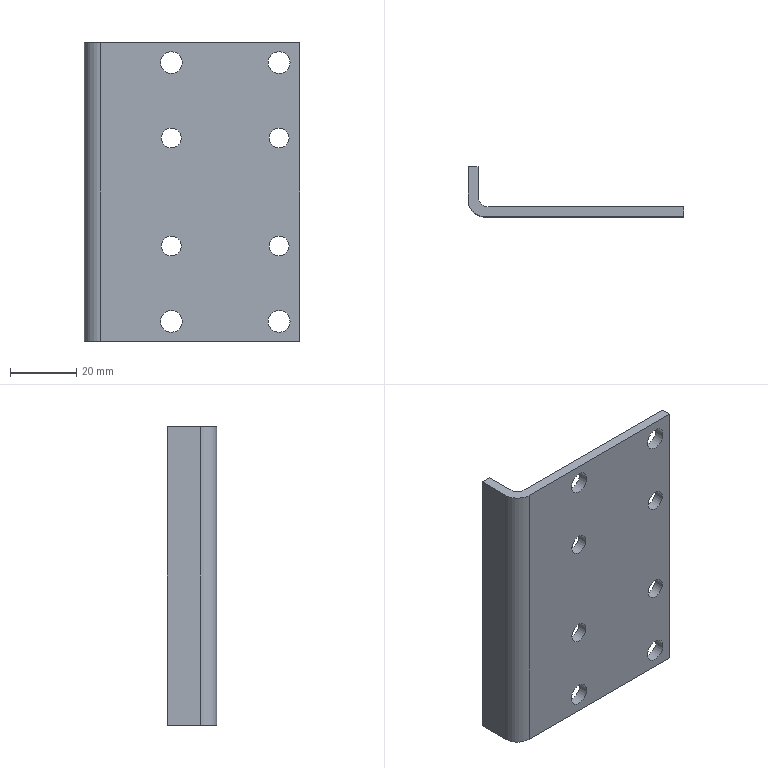Part | STEP file | wer4r34e | 1 solid | 18 faces | box 65 x 15 x 90 mm | volume 19731 mm3 | cylinder 10 | plane 8 | commonest cylinder face diameters 6 x5 6.6 x4 10 x1